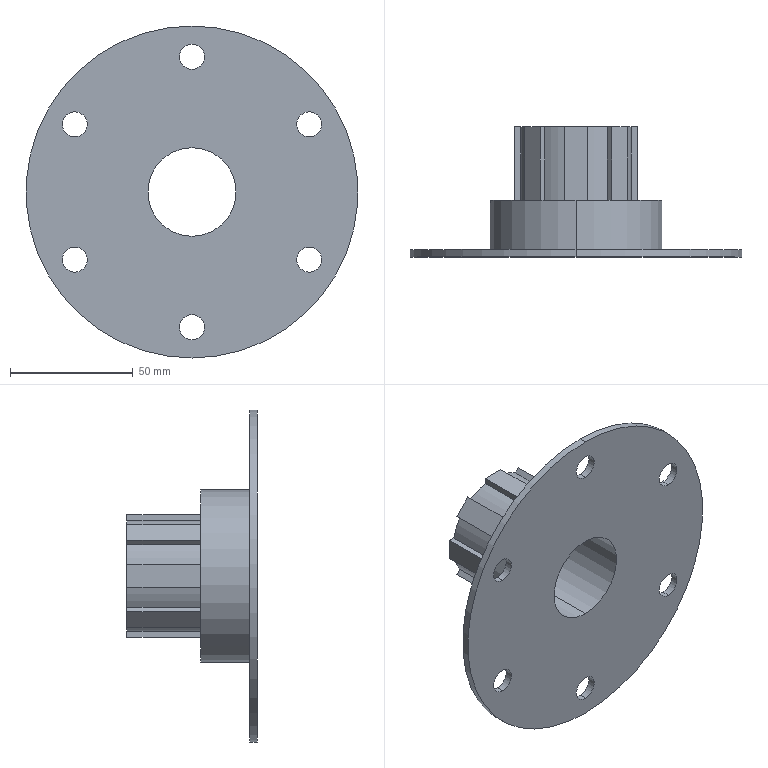Part | SolidWorks | features ICE 3, Extrusion 1, HoleWzd 1 | 1 solid | 54 faces | box 135 x 53 x 135 mm | volume 118988 mm3 | plane 28 | cylinder 26 | commonest cylinder face diameters 10.2 x12 46 x8 36 x2 70 x2 135 x2